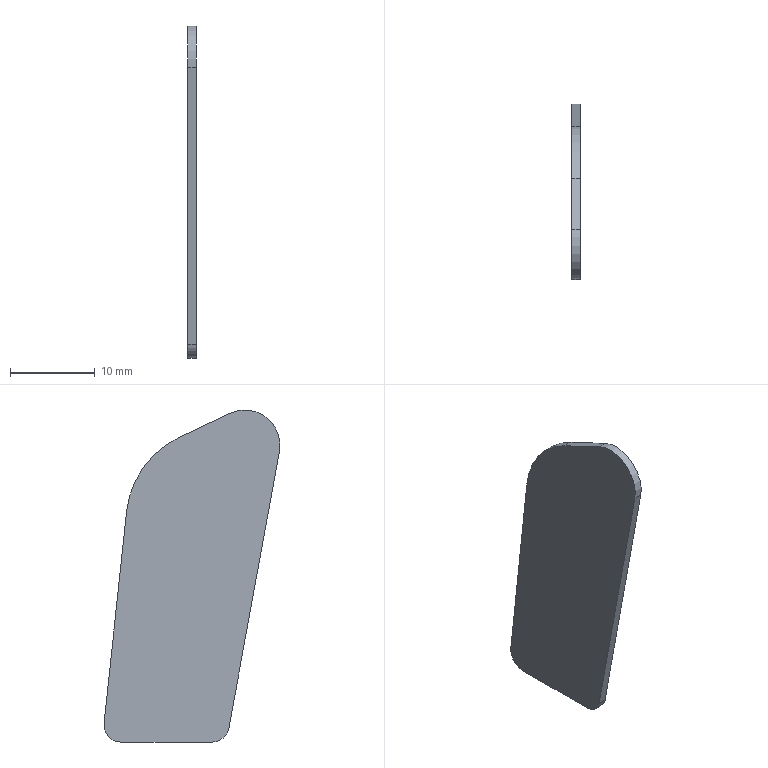Part | STEP file | 1-31.4 | 1 solid | 10 faces | box 1 x 20.769 x 39.162 mm | volume 584.948 mm3 | plane 6 | cylinder 4 | commonest cylinder face diameters 4 x2 8.325 x1 22 x1
STEP:
#1=CARTESIAN_POINT('',(0.,0.,0.));
#2=DIRECTION('',(0.,0.,1.));
#3=DIRECTION('',(1.,0.,0.));
#4=AXIS2_PLACEMENT_3D('',#1,#2,#3);
#5=CARTESIAN_POINT('',(0.,63.373,46.508));
#6=VERTEX_POINT('',#5);
#7=CARTESIAN_POINT('',(0.,57.49,42.001));
#8=VERTEX_POINT('',#7);
#9=CARTESIAN_POINT('',(0.,61.584,42.75));
#10=DIRECTION('',(1.,0.,0.));
#11=DIRECTION('',(0.,0.4297,0.903));
#12=AXIS2_PLACEMENT_3D('',#9,#10,#11);
#13=CIRCLE('',#12,4.162);
#14=CARTESIAN_POINT('',(0.,76.958,27.676));
#15=DIRECTION('',(1.,0.,0.));
#16=DIRECTION('',(0.,0.,-1.));
#17=AXIS2_PLACEMENT_3D('',#14,#15,#16);
#18=PLANE('',#17);
#19=CARTESIAN_POINT('',(-15.074,-15.374));
#20=DIRECTION('',(-0.903,0.4297));
#21=AXIS2_PLACEMENT_2D('',#19,#20);
#22=CIRCLE('',#21,4.162);
#23=(GEOMETRIC_REPRESENTATION_CONTEXT(2)PARAMETRIC_REPRESENTATION_CONTEXT()REPRESENTATION_CONTEXT('',''));
#24=DEFINITIONAL_REPRESENTATION('',(#22),#23);
#25=PCURVE('',#18,#24);
#26=CARTESIAN_POINT('',(0.,61.584,42.75));
#27=DIRECTION('',(-1.,0.,0.));
#28=DIRECTION('',(0.,0.4297,0.903));
#29=AXIS2_PLACEMENT_3D('',#26,#27,#28);
#30=CYLINDRICAL_SURFACE('',#29,4.162);
#31=CARTESIAN_POINT('',(6.283,0.));
#32=DIRECTION('',(-1.,0.));
#33=VECTOR('',#32,1.);
#34=LINE('',#31,#33);
#35=(GEOMETRIC_REPRESENTATION_CONTEXT(2)PARAMETRIC_REPRESENTATION_CONTEXT()REPRESENTATION_CONTEXT('',''));
#36=DEFINITIONAL_REPRESENTATION('',(#34),#35);
#37=PCURVE('',#30,#36);
#38=SURFACE_CURVE('',#13,(#25,#37),.PCURVE_S1.);
#39=EDGE_CURVE('',#6,#8,#38,.T.);
#40=ORIENTED_EDGE('',*,*,#39,.T.);
#41=CARTESIAN_POINT('',(0.,63.458,9.39));
#42=VERTEX_POINT('',#41);
#43=CARTESIAN_POINT('',(0.,57.49,42.001));
#44=DIRECTION('',(0.,0.18,-0.9837));
#45=VECTOR('',#44,1.);
#46=LINE('',#43,#45);
#47=CARTESIAN_POINT('',(-14.324,-19.468));
#48=DIRECTION('',(0.9837,0.18));
#49=VECTOR('',#48,1.);
#50=LINE('',#47,#49);
#51=(GEOMETRIC_REPRESENTATION_CONTEXT(2)PARAMETRIC_REPRESENTATION_CONTEXT()REPRESENTATION_CONTEXT('',''));
#52=DEFINITIONAL_REPRESENTATION('',(#50),#51);
#53=PCURVE('',#18,#52);
#54=CARTESIAN_POINT('',(-0.5,60.474,25.695));
#55=DIRECTION('',(0.,0.9837,0.18));
#56=DIRECTION('',(0.,0.18,-0.9837));
#57=AXIS2_PLACEMENT_3D('',#54,#55,#56);
#58=PLANE('',#57);
#59=CARTESIAN_POINT('',(-16.576,-0.5));
#60=DIRECTION('',(1.,0.));
#61=VECTOR('',#60,1.);
#62=LINE('',#59,#61);
#63=(GEOMETRIC_REPRESENTATION_CONTEXT(2)PARAMETRIC_REPRESENTATION_CONTEXT()REPRESENTATION_CONTEXT('',''));
#64=DEFINITIONAL_REPRESENTATION('',(#62),#63);
#65=PCURVE('',#58,#64);
#66=SURFACE_CURVE('',#46,(#53,#65),.PCURVE_S1.);
#67=EDGE_CURVE('',#8,#42,#66,.T.);
#68=ORIENTED_EDGE('',*,*,#67,.T.);
#69=CARTESIAN_POINT('',(0.,65.426,7.75));
#70=VERTEX_POINT('',#69);
#71=CARTESIAN_POINT('',(0.,65.426,9.75));
#72=DIRECTION('',(1.,0.,0.));
#73=DIRECTION('',(0.,-0.9837,-0.18));
#74=AXIS2_PLACEMENT_3D('',#71,#72,#73);
#75=CIRCLE('',#74,2.);
#76=CARTESIAN_POINT('',(17.926,-11.532));
#77=DIRECTION('',(0.18,-0.9837));
#78=AXIS2_PLACEMENT_2D('',#76,#77);
#79=CIRCLE('',#78,2.);
#80=(GEOMETRIC_REPRESENTATION_CONTEXT(2)PARAMETRIC_REPRESENTATION_CONTEXT()REPRESENTATION_CONTEXT('',''));
#81=DEFINITIONAL_REPRESENTATION('',(#79),#80);
#82=PCURVE('',#18,#81);
#83=CARTESIAN_POINT('',(0.,65.426,9.75));
#84=DIRECTION('',(-1.,0.,0.));
#85=DIRECTION('',(0.,-0.9837,-0.18));
#86=AXIS2_PLACEMENT_3D('',#83,#84,#85);
#87=CYLINDRICAL_SURFACE('',#86,2.);
#88=CARTESIAN_POINT('',(6.283,0.));
#89=DIRECTION('',(-1.,0.));
#90=VECTOR('',#89,1.);
#91=LINE('',#88,#90);
#92=(GEOMETRIC_REPRESENTATION_CONTEXT(2)PARAMETRIC_REPRESENTATION_CONTEXT()REPRESENTATION_CONTEXT('',''));
#93=DEFINITIONAL_REPRESENTATION('',(#91),#92);
#94=PCURVE('',#87,#93);
#95=SURFACE_CURVE('',#75,(#82,#94),.PCURVE_S1.);
#96=EDGE_CURVE('',#42,#70,#95,.T.);
#97=ORIENTED_EDGE('',*,*,#96,.T.);
#98=CARTESIAN_POINT('',(0.,76.191,7.75));
#99=VERTEX_POINT('',#98);
#100=CARTESIAN_POINT('',(0.,65.426,7.75));
#101=DIRECTION('',(0.,1.,0.));
#102=VECTOR('',#101,1.);
#103=LINE('',#100,#102);
#104=CARTESIAN_POINT('',(19.926,-11.532));
#105=DIRECTION('',(0.,1.));
#106=VECTOR('',#105,1.);
#107=LINE('',#104,#106);
#108=(GEOMETRIC_REPRESENTATION_CONTEXT(2)PARAMETRIC_REPRESENTATION_CONTEXT()REPRESENTATION_CONTEXT('',''));
#109=DEFINITIONAL_REPRESENTATION('',(#107),#108);
#110=PCURVE('',#18,#109);
#111=CARTESIAN_POINT('',(-0.5,70.808,7.75));
#112=DIRECTION('',(0.,0.,1.));
#113=DIRECTION('',(0.,1.,0.));
#114=AXIS2_PLACEMENT_3D('',#111,#112,#113);
#115=PLANE('',#114);
#116=CARTESIAN_POINT('',(-5.383,-0.5));
#117=DIRECTION('',(1.,0.));
#118=VECTOR('',#117,1.);
#119=LINE('',#116,#118);
#120=(GEOMETRIC_REPRESENTATION_CONTEXT(2)PARAMETRIC_REPRESENTATION_CONTEXT()REPRESENTATION_CONTEXT('',''));
#121=DEFINITIONAL_REPRESENTATION('',(#119),#120);
#122=PCURVE('',#115,#121);
#123=SURFACE_CURVE('',#103,(#110,#122),.PCURVE_S1.);
#124=EDGE_CURVE('',#70,#99,#123,.T.);
#125=ORIENTED_EDGE('',*,*,#124,.T.);
#126=CARTESIAN_POINT('',(0.,78.18,9.962));
#127=VERTEX_POINT('',#126);
#128=CARTESIAN_POINT('',(0.,76.191,9.75));
#129=DIRECTION('',(1.,0.,0.));
#130=DIRECTION('',(0.,0.,-1.));
#131=AXIS2_PLACEMENT_3D('',#128,#129,#130);
#132=CIRCLE('',#131,2.);
#133=CARTESIAN_POINT('',(17.926,-0.7664));
#134=DIRECTION('',(1.,0.));
#135=AXIS2_PLACEMENT_2D('',#133,#134);
#136=CIRCLE('',#135,2.);
#137=(GEOMETRIC_REPRESENTATION_CONTEXT(2)PARAMETRIC_REPRESENTATION_CONTEXT()REPRESENTATION_CONTEXT('',''));
#138=DEFINITIONAL_REPRESENTATION('',(#136),#137);
#139=PCURVE('',#18,#138);
#140=CARTESIAN_POINT('',(0.,76.191,9.75));
#141=DIRECTION('',(-1.,0.,0.));
#142=DIRECTION('',(0.,0.,-1.));
#143=AXIS2_PLACEMENT_3D('',#140,#141,#142);
#144=CYLINDRICAL_SURFACE('',#143,2.);
#145=CARTESIAN_POINT('',(6.283,0.));
#146=DIRECTION('',(-1.,0.));
#147=VECTOR('',#146,1.);
#148=LINE('',#145,#147);
#149=(GEOMETRIC_REPRESENTATION_CONTEXT(2)PARAMETRIC_REPRESENTATION_CONTEXT()REPRESENTATION_CONTEXT('',''));
#150=DEFINITIONAL_REPRESENTATION('',(#148),#149);
#151=PCURVE('',#144,#150);
#152=SURFACE_CURVE('',#132,(#139,#151),.PCURVE_S1.);
#153=EDGE_CURVE('',#99,#127,#152,.T.);
#154=ORIENTED_EDGE('',*,*,#153,.T.);
#155=CARTESIAN_POINT('',(0.,75.522,34.915));
#156=VERTEX_POINT('',#155);
#157=CARTESIAN_POINT('',(0.,78.18,9.962));
#158=DIRECTION('',(0.,-0.1059,0.9944));
#159=VECTOR('',#158,1.);
#160=LINE('',#157,#159);
#161=CARTESIAN_POINT('',(17.714,1.222));
#162=DIRECTION('',(-0.9944,-0.1059));
#163=VECTOR('',#162,1.);
#164=LINE('',#161,#163);
#165=(GEOMETRIC_REPRESENTATION_CONTEXT(2)PARAMETRIC_REPRESENTATION_CONTEXT()REPRESENTATION_CONTEXT('',''));
#166=DEFINITIONAL_REPRESENTATION('',(#164),#165);
#167=PCURVE('',#18,#166);
#168=CARTESIAN_POINT('',(-0.5,76.851,22.438));
#169=DIRECTION('',(0.,-0.9944,-0.1059));
#170=DIRECTION('',(0.,-0.1059,0.9944));
#171=AXIS2_PLACEMENT_3D('',#168,#169,#170);
#172=PLANE('',#171);
#173=CARTESIAN_POINT('',(-12.547,-0.5));
#174=DIRECTION('',(1.,0.));
#175=VECTOR('',#174,1.);
#176=LINE('',#173,#175);
#177=(GEOMETRIC_REPRESENTATION_CONTEXT(2)PARAMETRIC_REPRESENTATION_CONTEXT()REPRESENTATION_CONTEXT('',''));
#178=DEFINITIONAL_REPRESENTATION('',(#176),#177);
#179=PCURVE('',#172,#178);
#180=SURFACE_CURVE('',#160,(#167,#179),.PCURVE_S1.);
#181=EDGE_CURVE('',#127,#156,#180,.T.);
#182=ORIENTED_EDGE('',*,*,#181,.T.);
#183=CARTESIAN_POINT('',(0.,69.311,43.683));
#184=VERTEX_POINT('',#183);
#185=CARTESIAN_POINT('',(0.,64.584,33.75));
#186=DIRECTION('',(1.,0.,0.));
#187=DIRECTION('',(0.,0.9944,0.1059));
#188=AXIS2_PLACEMENT_3D('',#185,#186,#187);
#189=CIRCLE('',#188,11.);
#190=CARTESIAN_POINT('',(-6.074,-12.374));
#191=DIRECTION('',(-0.1059,0.9944));
#192=AXIS2_PLACEMENT_2D('',#190,#191);
#193=CIRCLE('',#192,11.);
#194=(GEOMETRIC_REPRESENTATION_CONTEXT(2)PARAMETRIC_REPRESENTATION_CONTEXT()REPRESENTATION_CONTEXT('',''));
#195=DEFINITIONAL_REPRESENTATION('',(#193),#194);
#196=PCURVE('',#18,#195);
#197=CARTESIAN_POINT('',(0.,64.584,33.75));
#198=DIRECTION('',(-1.,0.,0.));
#199=DIRECTION('',(0.,0.9944,0.1059));
#200=AXIS2_PLACEMENT_3D('',#197,#198,#199);
#201=CYLINDRICAL_SURFACE('',#200,11.);
#202=CARTESIAN_POINT('',(6.283,0.));
#203=DIRECTION('',(-1.,0.));
#204=VECTOR('',#203,1.);
#205=LINE('',#202,#204);
#206=(GEOMETRIC_REPRESENTATION_CONTEXT(2)PARAMETRIC_REPRESENTATION_CONTEXT()REPRESENTATION_CONTEXT('',''));
#207=DEFINITIONAL_REPRESENTATION('',(#205),#206);
#208=PCURVE('',#201,#207);
#209=SURFACE_CURVE('',#189,(#196,#208),.PCURVE_S1.);
#210=EDGE_CURVE('',#156,#184,#209,.T.);
#211=ORIENTED_EDGE('',*,*,#210,.T.);
#212=CARTESIAN_POINT('',(0.,69.311,43.683));
#213=DIRECTION('',(0.,-0.903,0.4297));
#214=VECTOR('',#213,1.);
#215=LINE('',#212,#214);
#216=CARTESIAN_POINT('',(-16.006,-7.647));
#217=DIRECTION('',(-0.4297,-0.903));
#218=VECTOR('',#217,1.);
#219=LINE('',#216,#218);
#220=(GEOMETRIC_REPRESENTATION_CONTEXT(2)PARAMETRIC_REPRESENTATION_CONTEXT()REPRESENTATION_CONTEXT('',''));
#221=DEFINITIONAL_REPRESENTATION('',(#219),#220);
#222=PCURVE('',#18,#221);
#223=CARTESIAN_POINT('',(-0.5,66.342,45.096));
#224=DIRECTION('',(0.,-0.4297,-0.903));
#225=DIRECTION('',(0.,-0.903,0.4297));
#226=AXIS2_PLACEMENT_3D('',#223,#224,#225);
#227=PLANE('',#226);
#228=CARTESIAN_POINT('',(-3.288,-0.5));
#229=DIRECTION('',(1.,0.));
#230=VECTOR('',#229,1.);
#231=LINE('',#228,#230);
#232=(GEOMETRIC_REPRESENTATION_CONTEXT(2)PARAMETRIC_REPRESENTATION_CONTEXT()REPRESENTATION_CONTEXT('',''));
#233=DEFINITIONAL_REPRESENTATION('',(#231),#232);
#234=PCURVE('',#227,#233);
#235=SURFACE_CURVE('',#215,(#222,#234),.PCURVE_S1.);
#236=EDGE_CURVE('',#184,#6,#235,.T.);
#237=ORIENTED_EDGE('',*,*,#236,.T.);
#238=EDGE_LOOP('',(#40,#68,#97,#125,#154,#182,#211,#237));
#239=FACE_BOUND('',#238,.T.);
#240=ADVANCED_FACE('',(#239),#18,.T.);
#241=CARTESIAN_POINT('',(-1.,63.373,46.508));
#242=VERTEX_POINT('',#241);
#243=CARTESIAN_POINT('',(-1.,57.49,42.001));
#244=VERTEX_POINT('',#243);
#245=CARTESIAN_POINT('',(-1.,61.584,42.75));
#246=DIRECTION('',(1.,0.,0.));
#247=DIRECTION('',(0.,0.4297,0.903));
#248=AXIS2_PLACEMENT_3D('',#245,#246,#247);
#249=CIRCLE('',#248,4.162);
#250=CARTESIAN_POINT('',(-1.,76.958,27.676));
#251=DIRECTION('',(1.,0.,0.));
#252=DIRECTION('',(0.,0.,-1.));
#253=AXIS2_PLACEMENT_3D('',#250,#251,#252);
#254=PLANE('',#253);
#255=CARTESIAN_POINT('',(-15.074,-15.374));
#256=DIRECTION('',(-0.903,0.4297));
#257=AXIS2_PLACEMENT_2D('',#255,#256);
#258=CIRCLE('',#257,4.162);
#259=(GEOMETRIC_REPRESENTATION_CONTEXT(2)PARAMETRIC_REPRESENTATION_CONTEXT()REPRESENTATION_CONTEXT('',''));
#260=DEFINITIONAL_REPRESENTATION('',(#258),#259);
#261=PCURVE('',#254,#260);
#262=CARTESIAN_POINT('',(6.283,1.));
#263=DIRECTION('',(-1.,0.));
#264=VECTOR('',#263,1.);
#265=LINE('',#262,#264);
#266=(GEOMETRIC_REPRESENTATION_CONTEXT(2)PARAMETRIC_REPRESENTATION_CONTEXT()REPRESENTATION_CONTEXT('',''));
#267=DEFINITIONAL_REPRESENTATION('',(#265),#266);
#268=PCURVE('',#30,#267);
#269=SURFACE_CURVE('',#249,(#261,#268),.PCURVE_S1.);
#270=EDGE_CURVE('',#242,#244,#269,.T.);
#271=ORIENTED_EDGE('',*,*,#270,.T.);
#272=CARTESIAN_POINT('',(-1.,63.458,9.39));
#273=VERTEX_POINT('',#272);
#274=CARTESIAN_POINT('',(-1.,57.49,42.001));
#275=DIRECTION('',(0.,0.18,-0.9837));
#276=VECTOR('',#275,1.);
#277=LINE('',#274,#276);
#278=CARTESIAN_POINT('',(-14.324,-19.468));
#279=DIRECTION('',(0.9837,0.18));
#280=VECTOR('',#279,1.);
#281=LINE('',#278,#280);
#282=(GEOMETRIC_REPRESENTATION_CONTEXT(2)PARAMETRIC_REPRESENTATION_CONTEXT()REPRESENTATION_CONTEXT('',''));
#283=DEFINITIONAL_REPRESENTATION('',(#281),#282);
#284=PCURVE('',#254,#283);
#285=CARTESIAN_POINT('',(-16.576,0.5));
#286=DIRECTION('',(1.,0.));
#287=VECTOR('',#286,1.);
#288=LINE('',#285,#287);
#289=(GEOMETRIC_REPRESENTATION_CONTEXT(2)PARAMETRIC_REPRESENTATION_CONTEXT()REPRESENTATION_CONTEXT('',''));
#290=DEFINITIONAL_REPRESENTATION('',(#288),#289);
#291=PCURVE('',#58,#290);
#292=SURFACE_CURVE('',#277,(#284,#291),.PCURVE_S1.);
#293=EDGE_CURVE('',#244,#273,#292,.T.);
#294=ORIENTED_EDGE('',*,*,#293,.T.);
#295=CARTESIAN_POINT('',(-1.,65.426,7.75));
#296=VERTEX_POINT('',#295);
#297=CARTESIAN_POINT('',(-1.,65.426,9.75));
#298=DIRECTION('',(1.,0.,0.));
#299=DIRECTION('',(0.,-0.9837,-0.18));
#300=AXIS2_PLACEMENT_3D('',#297,#298,#299);
#301=CIRCLE('',#300,2.);
#302=CARTESIAN_POINT('',(17.926,-11.532));
#303=DIRECTION('',(0.18,-0.9837));
#304=AXIS2_PLACEMENT_2D('',#302,#303);
#305=CIRCLE('',#304,2.);
#306=(GEOMETRIC_REPRESENTATION_CONTEXT(2)PARAMETRIC_REPRESENTATION_CONTEXT()REPRESENTATION_CONTEXT('',''));
#307=DEFINITIONAL_REPRESENTATION('',(#305),#306);
#308=PCURVE('',#254,#307);
#309=CARTESIAN_POINT('',(6.283,1.));
#310=DIRECTION('',(-1.,0.));
#311=VECTOR('',#310,1.);
#312=LINE('',#309,#311);
#313=(GEOMETRIC_REPRESENTATION_CONTEXT(2)PARAMETRIC_REPRESENTATION_CONTEXT()REPRESENTATION_CONTEXT('',''));
#314=DEFINITIONAL_REPRESENTATION('',(#312),#313);
#315=PCURVE('',#87,#314);
#316=SURFACE_CURVE('',#301,(#308,#315),.PCURVE_S1.);
#317=EDGE_CURVE('',#273,#296,#316,.T.);
#318=ORIENTED_EDGE('',*,*,#317,.T.);
#319=CARTESIAN_POINT('',(-1.,76.191,7.75));
#320=VERTEX_POINT('',#319);
#321=CARTESIAN_POINT('',(-1.,65.426,7.75));
#322=DIRECTION('',(0.,1.,0.));
#323=VECTOR('',#322,1.);
#324=LINE('',#321,#323);
#325=CARTESIAN_POINT('',(19.926,-11.532));
#326=DIRECTION('',(0.,1.));
#327=VECTOR('',#326,1.);
#328=LINE('',#325,#327);
#329=(GEOMETRIC_REPRESENTATION_CONTEXT(2)PARAMETRIC_REPRESENTATION_CONTEXT()REPRESENTATION_CONTEXT('',''));
#330=DEFINITIONAL_REPRESENTATION('',(#328),#329);
#331=PCURVE('',#254,#330);
#332=CARTESIAN_POINT('',(-5.383,0.5));
#333=DIRECTION('',(1.,0.));
#334=VECTOR('',#333,1.);
#335=LINE('',#332,#334);
#336=(GEOMETRIC_REPRESENTATION_CONTEXT(2)PARAMETRIC_REPRESENTATION_CONTEXT()REPRESENTATION_CONTEXT('',''));
#337=DEFINITIONAL_REPRESENTATION('',(#335),#336);
#338=PCURVE('',#115,#337);
#339=SURFACE_CURVE('',#324,(#331,#338),.PCURVE_S1.);
#340=EDGE_CURVE('',#296,#320,#339,.T.);
#341=ORIENTED_EDGE('',*,*,#340,.T.);
#342=CARTESIAN_POINT('',(-1.,78.18,9.962));
#343=VERTEX_POINT('',#342);
#344=CARTESIAN_POINT('',(-1.,76.191,9.75));
#345=DIRECTION('',(1.,0.,0.));
#346=DIRECTION('',(0.,0.,-1.));
#347=AXIS2_PLACEMENT_3D('',#344,#345,#346);
#348=CIRCLE('',#347,2.);
#349=CARTESIAN_POINT('',(17.926,-0.7664));
#350=DIRECTION('',(1.,0.));
#351=AXIS2_PLACEMENT_2D('',#349,#350);
#352=CIRCLE('',#351,2.);
#353=(GEOMETRIC_REPRESENTATION_CONTEXT(2)PARAMETRIC_REPRESENTATION_CONTEXT()REPRESENTATION_CONTEXT('',''));
#354=DEFINITIONAL_REPRESENTATION('',(#352),#353);
#355=PCURVE('',#254,#354);
#356=CARTESIAN_POINT('',(6.283,1.));
#357=DIRECTION('',(-1.,0.));
#358=VECTOR('',#357,1.);
#359=LINE('',#356,#358);
#360=(GEOMETRIC_REPRESENTATION_CONTEXT(2)PARAMETRIC_REPRESENTATION_CONTEXT()REPRESENTATION_CONTEXT('',''));
#361=DEFINITIONAL_REPRESENTATION('',(#359),#360);
#362=PCURVE('',#144,#361);
#363=SURFACE_CURVE('',#348,(#355,#362),.PCURVE_S1.);
#364=EDGE_CURVE('',#320,#343,#363,.T.);
#365=ORIENTED_EDGE('',*,*,#364,.T.);
#366=CARTESIAN_POINT('',(-1.,75.522,34.915));
#367=VERTEX_POINT('',#366);
#368=CARTESIAN_POINT('',(-1.,78.18,9.962));
#369=DIRECTION('',(0.,-0.1059,0.9944));
#370=VECTOR('',#369,1.);
#371=LINE('',#368,#370);
#372=CARTESIAN_POINT('',(17.714,1.222));
#373=DIRECTION('',(-0.9944,-0.1059));
#374=VECTOR('',#373,1.);
#375=LINE('',#372,#374);
#376=(GEOMETRIC_REPRESENTATION_CONTEXT(2)PARAMETRIC_REPRESENTATION_CONTEXT()REPRESENTATION_CONTEXT('',''));
#377=DEFINITIONAL_REPRESENTATION('',(#375),#376);
#378=PCURVE('',#254,#377);
#379=CARTESIAN_POINT('',(-12.547,0.5));
#380=DIRECTION('',(1.,0.));
#381=VECTOR('',#380,1.);
#382=LINE('',#379,#381);
#383=(GEOMETRIC_REPRESENTATION_CONTEXT(2)PARAMETRIC_REPRESENTATION_CONTEXT()REPRESENTATION_CONTEXT('',''));
#384=DEFINITIONAL_REPRESENTATION('',(#382),#383);
#385=PCURVE('',#172,#384);
#386=SURFACE_CURVE('',#371,(#378,#385),.PCURVE_S1.);
#387=EDGE_CURVE('',#343,#367,#386,.T.);
#388=ORIENTED_EDGE('',*,*,#387,.T.);
#389=CARTESIAN_POINT('',(-1.,69.311,43.683));
#390=VERTEX_POINT('',#389);
#391=CARTESIAN_POINT('',(-1.,64.584,33.75));
#392=DIRECTION('',(1.,0.,0.));
#393=DIRECTION('',(0.,0.9944,0.1059));
#394=AXIS2_PLACEMENT_3D('',#391,#392,#393);
#395=CIRCLE('',#394,11.);
#396=CARTESIAN_POINT('',(-6.074,-12.374));
#397=DIRECTION('',(-0.1059,0.9944));
#398=AXIS2_PLACEMENT_2D('',#396,#397);
#399=CIRCLE('',#398,11.);
#400=(GEOMETRIC_REPRESENTATION_CONTEXT(2)PARAMETRIC_REPRESENTATION_CONTEXT()REPRESENTATION_CONTEXT('',''));
#401=DEFINITIONAL_REPRESENTATION('',(#399),#400);
#402=PCURVE('',#254,#401);
#403=CARTESIAN_POINT('',(6.283,1.));
#404=DIRECTION('',(-1.,0.));
#405=VECTOR('',#404,1.);
#406=LINE('',#403,#405);
#407=(GEOMETRIC_REPRESENTATION_CONTEXT(2)PARAMETRIC_REPRESENTATION_CONTEXT()REPRESENTATION_CONTEXT('',''));
#408=DEFINITIONAL_REPRESENTATION('',(#406),#407);
#409=PCURVE('',#201,#408);
#410=SURFACE_CURVE('',#395,(#402,#409),.PCURVE_S1.);
#411=EDGE_CURVE('',#367,#390,#410,.T.);
#412=ORIENTED_EDGE('',*,*,#411,.T.);
#413=CARTESIAN_POINT('',(-1.,69.311,43.683));
#414=DIRECTION('',(0.,-0.903,0.4297));
#415=VECTOR('',#414,1.);
#416=LINE('',#413,#415);
#417=CARTESIAN_POINT('',(-16.006,-7.647));
#418=DIRECTION('',(-0.4297,-0.903));
#419=VECTOR('',#418,1.);
#420=LINE('',#417,#419);
#421=(GEOMETRIC_REPRESENTATION_CONTEXT(2)PARAMETRIC_REPRESENTATION_CONTEXT()REPRESENTATION_CONTEXT('',''));
#422=DEFINITIONAL_REPRESENTATION('',(#420),#421);
#423=PCURVE('',#254,#422);
#424=CARTESIAN_POINT('',(-3.288,0.5));
#425=DIRECTION('',(1.,0.));
#426=VECTOR('',#425,1.);
#427=LINE('',#424,#426);
#428=(GEOMETRIC_REPRESENTATION_CONTEXT(2)PARAMETRIC_REPRESENTATION_CONTEXT()REPRESENTATION_CONTEXT('',''));
#429=DEFINITIONAL_REPRESENTATION('',(#427),#428);
#430=PCURVE('',#227,#429);
#431=SURFACE_CURVE('',#416,(#423,#430),.PCURVE_S1.);
#432=EDGE_CURVE('',#390,#242,#431,.T.);
#433=ORIENTED_EDGE('',*,*,#432,.T.);
#434=EDGE_LOOP('',(#271,#294,#318,#341,#365,#388,#412,#433));
#435=FACE_BOUND('',#434,.F.);
#436=ADVANCED_FACE('',(#435),#254,.F.);
#437=CARTESIAN_POINT('',(0.,63.373,46.508));
#438=DIRECTION('',(-1.,0.,0.));
#439=VECTOR('',#438,1.);
#440=LINE('',#437,#439);
#441=CARTESIAN_POINT('',(6.283,0.));
#442=DIRECTION('',(0.,1.));
#443=VECTOR('',#442,1.);
#444=LINE('',#441,#443);
#445=(GEOMETRIC_REPRESENTATION_CONTEXT(2)PARAMETRIC_REPRESENTATION_CONTEXT()REPRESENTATION_CONTEXT('',''));
#446=DEFINITIONAL_REPRESENTATION('',(#444),#445);
#447=PCURVE('',#30,#446);
#448=CARTESIAN_POINT('',(3.288,-0.5));
#449=DIRECTION('',(0.,1.));
#450=VECTOR('',#449,1.);
#451=LINE('',#448,#450);
#452=(GEOMETRIC_REPRESENTATION_CONTEXT(2)PARAMETRIC_REPRESENTATION_CONTEXT()REPRESENTATION_CONTEXT('',''));
#453=DEFINITIONAL_REPRESENTATION('',(#451),#452);
#454=PCURVE('',#227,#453);
#455=SURFACE_CURVE('',#440,(#447,#454),.PCURVE_S1.);
#456=EDGE_CURVE('',#6,#242,#455,.T.);
#457=ORIENTED_EDGE('',*,*,#456,.T.);
#458=ORIENTED_EDGE('',*,*,#270,.T.);
#459=CARTESIAN_POINT('',(0.,57.49,42.001));
#460=DIRECTION('',(-1.,0.,0.));
#461=VECTOR('',#460,1.);
#462=LINE('',#459,#461);
#463=CARTESIAN_POINT('',(4.087,0.));
#464=DIRECTION('',(0.,1.));
#465=VECTOR('',#464,1.);
#466=LINE('',#463,#465);
#467=(GEOMETRIC_REPRESENTATION_CONTEXT(2)PARAMETRIC_REPRESENTATION_CONTEXT()REPRESENTATION_CONTEXT('',''));
#468=DEFINITIONAL_REPRESENTATION('',(#466),#467);
#469=PCURVE('',#30,#468);
#470=CARTESIAN_POINT('',(-16.576,-0.5));
#471=DIRECTION('',(0.,1.));
#472=VECTOR('',#471,1.);
#473=LINE('',#470,#472);
#474=(GEOMETRIC_REPRESENTATION_CONTEXT(2)PARAMETRIC_REPRESENTATION_CONTEXT()REPRESENTATION_CONTEXT('',''));
#475=DEFINITIONAL_REPRESENTATION('',(#473),#474);
#476=PCURVE('',#58,#475);
#477=SURFACE_CURVE('',#462,(#469,#476),.PCURVE_S1.);
#478=EDGE_CURVE('',#8,#244,#477,.T.);
#479=ORIENTED_EDGE('',*,*,#478,.F.);
#480=ORIENTED_EDGE('',*,*,#39,.F.);
#481=EDGE_LOOP('',(#457,#458,#479,#480));
#482=FACE_BOUND('',#481,.T.);
#483=ADVANCED_FACE('',(#482),#30,.T.);
#484=ORIENTED_EDGE('',*,*,#67,.T.);
#485=CARTESIAN_POINT('',(0.,63.458,9.39));
#486=DIRECTION('',(-1.,0.,0.));
#487=VECTOR('',#486,1.);
#488=LINE('',#485,#487);
#489=CARTESIAN_POINT('',(16.576,-0.5));
#490=DIRECTION('',(0.,1.));
#491=VECTOR('',#490,1.);
#492=LINE('',#489,#491);
#493=(GEOMETRIC_REPRESENTATION_CONTEXT(2)PARAMETRIC_REPRESENTATION_CONTEXT()REPRESENTATION_CONTEXT('',''));
#494=DEFINITIONAL_REPRESENTATION('',(#492),#493);
#495=PCURVE('',#58,#494);
#496=CARTESIAN_POINT('',(6.283,0.));
#497=DIRECTION('',(0.,1.));
#498=VECTOR('',#497,1.);
#499=LINE('',#496,#498);
#500=(GEOMETRIC_REPRESENTATION_CONTEXT(2)PARAMETRIC_REPRESENTATION_CONTEXT()REPRESENTATION_CONTEXT('',''));
#501=DEFINITIONAL_REPRESENTATION('',(#499),#500);
#502=PCURVE('',#87,#501);
#503=SURFACE_CURVE('',#488,(#495,#502),.PCURVE_S1.);
#504=EDGE_CURVE('',#42,#273,#503,.T.);
#505=ORIENTED_EDGE('',*,*,#504,.T.);
#506=ORIENTED_EDGE('',*,*,#293,.F.);
#507=ORIENTED_EDGE('',*,*,#478,.F.);
#508=EDGE_LOOP('',(#484,#505,#506,#507));
#509=FACE_BOUND('',#508,.F.);
#510=ADVANCED_FACE('',(#509),#58,.F.);
#511=ORIENTED_EDGE('',*,*,#504,.T.);
#512=ORIENTED_EDGE('',*,*,#317,.T.);
#513=CARTESIAN_POINT('',(0.,65.426,7.75));
#514=DIRECTION('',(-1.,0.,0.));
#515=VECTOR('',#514,1.);
#516=LINE('',#513,#515);
#517=CARTESIAN_POINT('',(4.893,0.));
#518=DIRECTION('',(0.,1.));
#519=VECTOR('',#518,1.);
#520=LINE('',#517,#519);
#521=(GEOMETRIC_REPRESENTATION_CONTEXT(2)PARAMETRIC_REPRESENTATION_CONTEXT()REPRESENTATION_CONTEXT('',''));
#522=DEFINITIONAL_REPRESENTATION('',(#520),#521);
#523=PCURVE('',#87,#522);
#524=CARTESIAN_POINT('',(-5.383,-0.5));
#525=DIRECTION('',(0.,1.));
#526=VECTOR('',#525,1.);
#527=LINE('',#524,#526);
#528=(GEOMETRIC_REPRESENTATION_CONTEXT(2)PARAMETRIC_REPRESENTATION_CONTEXT()REPRESENTATION_CONTEXT('',''));
#529=DEFINITIONAL_REPRESENTATION('',(#527),#528);
#530=PCURVE('',#115,#529);
#531=SURFACE_CURVE('',#516,(#523,#530),.PCURVE_S1.);
#532=EDGE_CURVE('',#70,#296,#531,.T.);
#533=ORIENTED_EDGE('',*,*,#532,.F.);
#534=ORIENTED_EDGE('',*,*,#96,.F.);
#535=EDGE_LOOP('',(#511,#512,#533,#534));
#536=FACE_BOUND('',#535,.T.);
#537=ADVANCED_FACE('',(#536),#87,.T.);
#538=ORIENTED_EDGE('',*,*,#124,.T.);
#539=CARTESIAN_POINT('',(0.,76.191,7.75));
#540=DIRECTION('',(-1.,0.,0.));
#541=VECTOR('',#540,1.);
#542=LINE('',#539,#541);
#543=CARTESIAN_POINT('',(5.383,-0.5));
#544=DIRECTION('',(0.,1.));
#545=VECTOR('',#544,1.);
#546=LINE('',#543,#545);
#547=(GEOMETRIC_REPRESENTATION_CONTEXT(2)PARAMETRIC_REPRESENTATION_CONTEXT()REPRESENTATION_CONTEXT('',''));
#548=DEFINITIONAL_REPRESENTATION('',(#546),#547);
#549=PCURVE('',#115,#548);
#550=CARTESIAN_POINT('',(6.283,0.));
#551=DIRECTION('',(0.,1.));
#552=VECTOR('',#551,1.);
#553=LINE('',#550,#552);
#554=(GEOMETRIC_REPRESENTATION_CONTEXT(2)PARAMETRIC_REPRESENTATION_CONTEXT()REPRESENTATION_CONTEXT('',''));
#555=DEFINITIONAL_REPRESENTATION('',(#553),#554);
#556=PCURVE('',#144,#555);
#557=SURFACE_CURVE('',#542,(#549,#556),.PCURVE_S1.);
#558=EDGE_CURVE('',#99,#320,#557,.T.);
#559=ORIENTED_EDGE('',*,*,#558,.T.);
#560=ORIENTED_EDGE('',*,*,#340,.F.);
#561=ORIENTED_EDGE('',*,*,#532,.F.);
#562=EDGE_LOOP('',(#538,#559,#560,#561));
#563=FACE_BOUND('',#562,.F.);
#564=ADVANCED_FACE('',(#563),#115,.F.);
#565=ORIENTED_EDGE('',*,*,#558,.T.);
#566=ORIENTED_EDGE('',*,*,#364,.T.);
#567=CARTESIAN_POINT('',(0.,78.18,9.962));
#568=DIRECTION('',(-1.,0.,0.));
#569=VECTOR('',#568,1.);
#570=LINE('',#567,#569);
#571=CARTESIAN_POINT('',(4.606,0.));
#572=DIRECTION('',(0.,1.));
#573=VECTOR('',#572,1.);
#574=LINE('',#571,#573);
#575=(GEOMETRIC_REPRESENTATION_CONTEXT(2)PARAMETRIC_REPRESENTATION_CONTEXT()REPRESENTATION_CONTEXT('',''));
#576=DEFINITIONAL_REPRESENTATION('',(#574),#575);
#577=PCURVE('',#144,#576);
#578=CARTESIAN_POINT('',(-12.547,-0.5));
#579=DIRECTION('',(0.,1.));
#580=VECTOR('',#579,1.);
#581=LINE('',#578,#580);
#582=(GEOMETRIC_REPRESENTATION_CONTEXT(2)PARAMETRIC_REPRESENTATION_CONTEXT()REPRESENTATION_CONTEXT('',''));
#583=DEFINITIONAL_REPRESENTATION('',(#581),#582);
#584=PCURVE('',#172,#583);
#585=SURFACE_CURVE('',#570,(#577,#584),.PCURVE_S1.);
#586=EDGE_CURVE('',#127,#343,#585,.T.);
#587=ORIENTED_EDGE('',*,*,#586,.F.);
#588=ORIENTED_EDGE('',*,*,#153,.F.);
#589=EDGE_LOOP('',(#565,#566,#587,#588));
#590=FACE_BOUND('',#589,.T.);
#591=ADVANCED_FACE('',(#590),#144,.T.);
#592=ORIENTED_EDGE('',*,*,#181,.T.);
#593=CARTESIAN_POINT('',(0.,75.522,34.915));
#594=DIRECTION('',(-1.,0.,0.));
#595=VECTOR('',#594,1.);
#596=LINE('',#593,#595);
#597=CARTESIAN_POINT('',(12.547,-0.5));
#598=DIRECTION('',(0.,1.));
#599=VECTOR('',#598,1.);
#600=LINE('',#597,#599);
#601=(GEOMETRIC_REPRESENTATION_CONTEXT(2)PARAMETRIC_REPRESENTATION_CONTEXT()REPRESENTATION_CONTEXT('',''));
#602=DEFINITIONAL_REPRESENTATION('',(#600),#601);
#603=PCURVE('',#172,#602);
#604=CARTESIAN_POINT('',(6.283,0.));
#605=DIRECTION('',(0.,1.));
#606=VECTOR('',#605,1.);
#607=LINE('',#604,#606);
#608=(GEOMETRIC_REPRESENTATION_CONTEXT(2)PARAMETRIC_REPRESENTATION_CONTEXT()REPRESENTATION_CONTEXT('',''));
#609=DEFINITIONAL_REPRESENTATION('',(#607),#608);
#610=PCURVE('',#201,#609);
#611=SURFACE_CURVE('',#596,(#603,#610),.PCURVE_S1.);
#612=EDGE_CURVE('',#156,#367,#611,.T.);
#613=ORIENTED_EDGE('',*,*,#612,.T.);
#614=ORIENTED_EDGE('',*,*,#387,.F.);
#615=ORIENTED_EDGE('',*,*,#586,.F.);
#616=EDGE_LOOP('',(#592,#613,#614,#615));
#617=FACE_BOUND('',#616,.F.);
#618=ADVANCED_FACE('',(#617),#172,.F.);
#619=ORIENTED_EDGE('',*,*,#612,.T.);
#620=ORIENTED_EDGE('',*,*,#411,.T.);
#621=CARTESIAN_POINT('',(0.,69.311,43.683));
#622=DIRECTION('',(-1.,0.,0.));
#623=VECTOR('',#622,1.);
#624=LINE('',#621,#623);
#625=CARTESIAN_POINT('',(5.263,0.));
#626=DIRECTION('',(0.,1.));
#627=VECTOR('',#626,1.);
#628=LINE('',#625,#627);
#629=(GEOMETRIC_REPRESENTATION_CONTEXT(2)PARAMETRIC_REPRESENTATION_CONTEXT()REPRESENTATION_CONTEXT('',''));
#630=DEFINITIONAL_REPRESENTATION('',(#628),#629);
#631=PCURVE('',#201,#630);
#632=CARTESIAN_POINT('',(-3.288,-0.5));
#633=DIRECTION('',(0.,1.));
#634=VECTOR('',#633,1.);
#635=LINE('',#632,#634);
#636=(GEOMETRIC_REPRESENTATION_CONTEXT(2)PARAMETRIC_REPRESENTATION_CONTEXT()REPRESENTATION_CONTEXT('',''));
#637=DEFINITIONAL_REPRESENTATION('',(#635),#636);
#638=PCURVE('',#227,#637);
#639=SURFACE_CURVE('',#624,(#631,#638),.PCURVE_S1.);
#640=EDGE_CURVE('',#184,#390,#639,.T.);
#641=ORIENTED_EDGE('',*,*,#640,.F.);
#642=ORIENTED_EDGE('',*,*,#210,.F.);
#643=EDGE_LOOP('',(#619,#620,#641,#642));
#644=FACE_BOUND('',#643,.T.);
#645=ADVANCED_FACE('',(#644),#201,.T.);
#646=ORIENTED_EDGE('',*,*,#236,.T.);
#647=ORIENTED_EDGE('',*,*,#456,.T.);
#648=ORIENTED_EDGE('',*,*,#432,.F.);
#649=ORIENTED_EDGE('',*,*,#640,.F.);
#650=EDGE_LOOP('',(#646,#647,#648,#649));
#651=FACE_BOUND('',#650,.F.);
#652=ADVANCED_FACE('',(#651),#227,.F.);
#653=CLOSED_SHELL('',(#240,#436,#483,#510,#537,#564,#591,#618,#645,#652));
#654=MANIFOLD_SOLID_BREP('',#653);
#655=(LENGTH_UNIT()NAMED_UNIT(*)SI_UNIT(.MILLI.,.METRE.));
#656=UNCERTAINTY_MEASURE_WITH_UNIT(LENGTH_MEASURE(0.0000001),#655,'','');
#657=(NAMED_UNIT(*)PLANE_ANGLE_UNIT()SI_UNIT($,.RADIAN.));
#658=(NAMED_UNIT(*)SI_UNIT($,.STERADIAN.)SOLID_ANGLE_UNIT());
#659=(GEOMETRIC_REPRESENTATION_CONTEXT(3)GLOBAL_UNCERTAINTY_ASSIGNED_CONTEXT((#656))GLOBAL_UNIT_ASSIGNED_CONTEXT((#655,#657,#658))REPRESENTATION_CONTEXT('',''));
#660=ADVANCED_BREP_SHAPE_REPRESENTATION('',(#4,#654),#659);